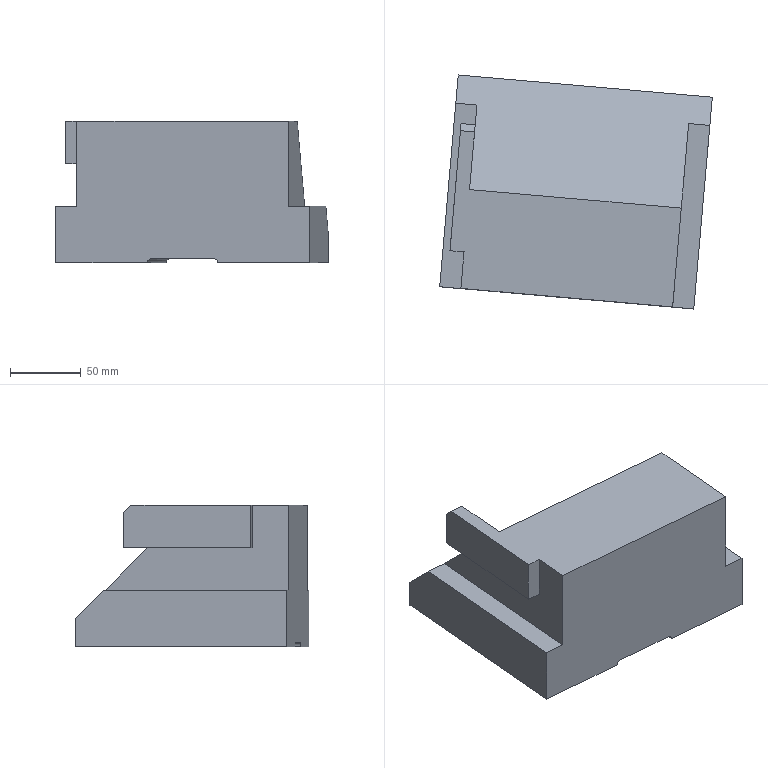Part | NX | features MAIN_BODY 2 | 1 solid | 21 faces | box 192.388 x 165.117 x 100 mm | volume 1948955 mm3 | plane 19 | cylinder 2 | commonest cylinder face diameters 6 x2
STEP:
#1=CARTESIAN_POINT('',(313.562,199.287,40.));
#2=VERTEX_POINT('',#1);
#3=CARTESIAN_POINT('',(306.154,114.611,40.));
#4=VERTEX_POINT('',#3);
#5=CARTESIAN_POINT('',(313.562,199.287,40.));
#6=CARTESIAN_POINT('',(311.093,171.062,40.));
#7=CARTESIAN_POINT('',(308.623,142.836,40.));
#8=CARTESIAN_POINT('',(306.154,114.611,40.));
#9=B_SPLINE_CURVE_WITH_KNOTS('',3,(#5,#6,#7,#8),.UNSPECIFIED.,.F.,.F.,(4,4),(0.,1.),.UNSPECIFIED.);
#10=EDGE_CURVE('',#2,#4,#9,.T.);
#11=ORIENTED_EDGE('',*,*,#10,.T.);
#12=CARTESIAN_POINT('',(316.116,113.739,40.));
#13=VERTEX_POINT('',#12);
#14=CARTESIAN_POINT('',(306.154,114.611,40.));
#15=CARTESIAN_POINT('',(309.475,114.32,40.));
#16=CARTESIAN_POINT('',(312.795,114.03,40.));
#17=CARTESIAN_POINT('',(316.116,113.739,40.));
#18=B_SPLINE_CURVE_WITH_KNOTS('',3,(#14,#15,#16,#17),.UNSPECIFIED.,.F.,.F.,(4,4),(0.,1.),.UNSPECIFIED.);
#19=EDGE_CURVE('',#4,#13,#18,.T.);
#20=ORIENTED_EDGE('',*,*,#19,.T.);
#21=CARTESIAN_POINT('',(313.862,87.98,40.));
#22=VERTEX_POINT('',#21);
#23=CARTESIAN_POINT('',(316.116,113.739,40.));
#24=CARTESIAN_POINT('',(315.365,105.153,40.));
#25=CARTESIAN_POINT('',(314.614,96.566,40.));
#26=CARTESIAN_POINT('',(313.862,87.98,40.));
#27=B_SPLINE_CURVE_WITH_KNOTS('',3,(#23,#24,#25,#26),.UNSPECIFIED.,.F.,.F.,(4,4),(0.,1.),.UNSPECIFIED.);
#28=EDGE_CURVE('',#13,#22,#27,.T.);
#29=ORIENTED_EDGE('',*,*,#28,.T.);
#30=CARTESIAN_POINT('',(463.291,74.907,40.));
#31=VERTEX_POINT('',#30);
#32=CARTESIAN_POINT('',(313.862,87.98,40.));
#33=CARTESIAN_POINT('',(363.672,83.622,40.));
#34=CARTESIAN_POINT('',(413.482,79.264,40.));
#35=CARTESIAN_POINT('',(463.291,74.907,40.));
#36=B_SPLINE_CURVE_WITH_KNOTS('',3,(#32,#33,#34,#35),.UNSPECIFIED.,.F.,.F.,(4,4),(0.,1.),.UNSPECIFIED.);
#37=EDGE_CURVE('',#22,#31,#36,.T.);
#38=ORIENTED_EDGE('',*,*,#37,.T.);
#39=CARTESIAN_POINT('',(469.392,144.64,40.));
#40=VERTEX_POINT('',#39);
#41=CARTESIAN_POINT('',(463.291,74.907,40.));
#42=CARTESIAN_POINT('',(465.325,98.151,40.));
#43=CARTESIAN_POINT('',(467.359,121.396,40.));
#44=CARTESIAN_POINT('',(469.392,144.64,40.));
#45=B_SPLINE_CURVE_WITH_KNOTS('',3,(#41,#42,#43,#44),.UNSPECIFIED.,.F.,.F.,(4,4),(0.,1.),.UNSPECIFIED.);
#46=EDGE_CURVE('',#31,#40,#45,.T.);
#47=ORIENTED_EDGE('',*,*,#46,.T.);
#48=CARTESIAN_POINT('',(319.963,157.714,40.));
#49=VERTEX_POINT('',#48);
#50=CARTESIAN_POINT('',(469.392,144.64,40.));
#51=CARTESIAN_POINT('',(419.583,148.998,40.));
#52=CARTESIAN_POINT('',(369.773,153.356,40.));
#53=CARTESIAN_POINT('',(319.963,157.714,40.));
#54=B_SPLINE_CURVE_WITH_KNOTS('',3,(#50,#51,#52,#53),.UNSPECIFIED.,.F.,.F.,(4,4),(0.,1.),.UNSPECIFIED.);
#55=EDGE_CURVE('',#40,#49,#54,.T.);
#56=ORIENTED_EDGE('',*,*,#55,.T.);
#57=CARTESIAN_POINT('',(323.524,198.416,40.));
#58=VERTEX_POINT('',#57);
#59=CARTESIAN_POINT('',(319.963,157.714,40.));
#60=CARTESIAN_POINT('',(321.15,171.281,40.));
#61=CARTESIAN_POINT('',(322.337,184.848,40.));
#62=CARTESIAN_POINT('',(323.524,198.416,40.));
#63=B_SPLINE_CURVE_WITH_KNOTS('',3,(#59,#60,#61,#62),.UNSPECIFIED.,.F.,.F.,(4,4),(0.,1.),.UNSPECIFIED.);
#64=EDGE_CURVE('',#49,#58,#63,.T.);
#65=ORIENTED_EDGE('',*,*,#64,.T.);
#66=CARTESIAN_POINT('',(323.524,198.416,40.));
#67=CARTESIAN_POINT('',(320.204,198.706,40.));
#68=CARTESIAN_POINT('',(316.883,198.997,40.));
#69=CARTESIAN_POINT('',(313.562,199.287,40.));
#70=B_SPLINE_CURVE_WITH_KNOTS('',3,(#66,#67,#68,#69),.UNSPECIFIED.,.F.,.F.,(4,4),(0.,1.),.UNSPECIFIED.);
#71=EDGE_CURVE('',#58,#2,#70,.T.);
#72=ORIENTED_EDGE('',*,*,#71,.T.);
#73=EDGE_LOOP('',(#11,#20,#29,#38,#47,#56,#65,#72));
#74=FACE_BOUND('',#73,.T.);
#75=CARTESIAN_POINT('',(388.427,137.097,40.));
#76=DIRECTION('',(0.,0.,1.));
#77=DIRECTION('',(-0.9962,0.08716,0.));
#78=AXIS2_PLACEMENT_3D('',#75,#76,#77);
#79=PLANE('',#78);
#80=ADVANCED_FACE('',(#74),#79,.T.);
#81=CARTESIAN_POINT('',(316.116,113.739,10.));
#82=VERTEX_POINT('',#81);
#83=CARTESIAN_POINT('',(316.116,113.739,10.));
#84=CARTESIAN_POINT('',(316.116,113.739,20.));
#85=CARTESIAN_POINT('',(316.116,113.739,30.));
#86=CARTESIAN_POINT('',(316.116,113.739,40.));
#87=B_SPLINE_CURVE_WITH_KNOTS('',3,(#83,#84,#85,#86),.UNSPECIFIED.,.F.,.F.,(4,4),(0.,1.),.UNSPECIFIED.);
#88=EDGE_CURVE('',#82,#13,#87,.T.);
#89=ORIENTED_EDGE('',*,*,#88,.T.);
#90=ORIENTED_EDGE('',*,*,#19,.F.);
#91=CARTESIAN_POINT('',(306.154,114.611,10.));
#92=VERTEX_POINT('',#91);
#93=CARTESIAN_POINT('',(306.154,114.611,40.));
#94=CARTESIAN_POINT('',(306.154,114.611,30.));
#95=CARTESIAN_POINT('',(306.154,114.611,20.));
#96=CARTESIAN_POINT('',(306.154,114.611,10.));
#97=B_SPLINE_CURVE_WITH_KNOTS('',3,(#93,#94,#95,#96),.UNSPECIFIED.,.F.,.F.,(4,4),(0.,1.),.UNSPECIFIED.);
#98=EDGE_CURVE('',#4,#92,#97,.T.);
#99=ORIENTED_EDGE('',*,*,#98,.T.);
#100=CARTESIAN_POINT('',(306.154,114.611,10.));
#101=CARTESIAN_POINT('',(309.475,114.32,10.));
#102=CARTESIAN_POINT('',(312.795,114.03,10.));
#103=CARTESIAN_POINT('',(316.116,113.739,10.));
#104=B_SPLINE_CURVE_WITH_KNOTS('',3,(#100,#101,#102,#103),.UNSPECIFIED.,.F.,.F.,(4,4),(0.,1.),.UNSPECIFIED.);
#105=EDGE_CURVE('',#92,#82,#104,.T.);
#106=ORIENTED_EDGE('',*,*,#105,.T.);
#107=EDGE_LOOP('',(#89,#90,#99,#106));
#108=FACE_BOUND('',#107,.T.);
#109=CARTESIAN_POINT('',(311.135,114.175,25.));
#110=DIRECTION('',(-0.08716,-0.9962,0.));
#111=DIRECTION('',(0.9962,-0.08716,0.));
#112=AXIS2_PLACEMENT_3D('',#109,#110,#111);
#113=PLANE('',#112);
#114=ADVANCED_FACE('',(#108),#113,.T.);
#115=CARTESIAN_POINT('',(313.998,204.268,10.));
#116=VERTEX_POINT('',#115);
#117=CARTESIAN_POINT('',(313.998,204.268,10.));
#118=CARTESIAN_POINT('',(311.383,174.383,10.));
#119=CARTESIAN_POINT('',(308.769,144.497,10.));
#120=CARTESIAN_POINT('',(306.154,114.611,10.));
#121=B_SPLINE_CURVE_WITH_KNOTS('',3,(#117,#118,#119,#120),.UNSPECIFIED.,.F.,.F.,(4,4),(0.,1.),.UNSPECIFIED.);
#122=EDGE_CURVE('',#116,#92,#121,.T.);
#123=ORIENTED_EDGE('',*,*,#122,.T.);
#124=ORIENTED_EDGE('',*,*,#98,.F.);
#125=ORIENTED_EDGE('',*,*,#10,.F.);
#126=CARTESIAN_POINT('',(313.998,204.268,35.));
#127=VERTEX_POINT('',#126);
#128=CARTESIAN_POINT('',(313.562,199.287,40.));
#129=CARTESIAN_POINT('',(313.708,200.948,38.333));
#130=CARTESIAN_POINT('',(313.853,202.608,36.667));
#131=CARTESIAN_POINT('',(313.998,204.268,35.));
#132=B_SPLINE_CURVE_WITH_KNOTS('',3,(#128,#129,#130,#131),.UNSPECIFIED.,.F.,.F.,(4,4),(0.,1.),.UNSPECIFIED.);
#133=EDGE_CURVE('',#2,#127,#132,.T.);
#134=ORIENTED_EDGE('',*,*,#133,.T.);
#135=CARTESIAN_POINT('',(313.998,204.268,35.));
#136=CARTESIAN_POINT('',(313.998,204.268,26.667));
#137=CARTESIAN_POINT('',(313.998,204.268,18.333));
#138=CARTESIAN_POINT('',(313.998,204.268,10.));
#139=B_SPLINE_CURVE_WITH_KNOTS('',3,(#135,#136,#137,#138),.UNSPECIFIED.,.F.,.F.,(4,4),(0.,1.),.UNSPECIFIED.);
#140=EDGE_CURVE('',#127,#116,#139,.T.);
#141=ORIENTED_EDGE('',*,*,#140,.T.);
#142=EDGE_LOOP('',(#123,#124,#125,#134,#141));
#143=FACE_BOUND('',#142,.T.);
#144=CARTESIAN_POINT('',(310.076,159.44,25.));
#145=DIRECTION('',(-0.9962,0.08716,0.));
#146=DIRECTION('',(-0.08716,-0.9962,0.));
#147=AXIS2_PLACEMENT_3D('',#144,#145,#146);
#148=PLANE('',#147);
#149=ADVANCED_FACE('',(#143),#148,.T.);
#150=CARTESIAN_POINT('',(323.96,203.397,35.));
#151=VERTEX_POINT('',#150);
#152=CARTESIAN_POINT('',(323.524,198.416,40.));
#153=CARTESIAN_POINT('',(323.669,200.076,38.333));
#154=CARTESIAN_POINT('',(323.815,201.737,36.667));
#155=CARTESIAN_POINT('',(323.96,203.397,35.));
#156=B_SPLINE_CURVE_WITH_KNOTS('',3,(#152,#153,#154,#155),.UNSPECIFIED.,.F.,.F.,(4,4),(0.,1.),.UNSPECIFIED.);
#157=EDGE_CURVE('',#58,#151,#156,.T.);
#158=ORIENTED_EDGE('',*,*,#157,.T.);
#159=CARTESIAN_POINT('',(323.96,203.397,35.));
#160=CARTESIAN_POINT('',(320.639,203.687,35.));
#161=CARTESIAN_POINT('',(317.319,203.978,35.));
#162=CARTESIAN_POINT('',(313.998,204.268,35.));
#163=B_SPLINE_CURVE_WITH_KNOTS('',3,(#159,#160,#161,#162),.UNSPECIFIED.,.F.,.F.,(4,4),(0.,1.),.UNSPECIFIED.);
#164=EDGE_CURVE('',#151,#127,#163,.T.);
#165=ORIENTED_EDGE('',*,*,#164,.T.);
#166=ORIENTED_EDGE('',*,*,#133,.F.);
#167=ORIENTED_EDGE('',*,*,#71,.F.);
#168=EDGE_LOOP('',(#158,#165,#166,#167));
#169=FACE_BOUND('',#168,.T.);
#170=CARTESIAN_POINT('',(318.761,201.342,37.5));
#171=DIRECTION('',(0.06163,0.7044,0.7071));
#172=DIRECTION('',(0.06163,0.7044,-0.7071));
#173=AXIS2_PLACEMENT_3D('',#170,#171,#172);
#174=PLANE('',#173);
#175=ADVANCED_FACE('',(#169),#174,.T.);
#176=ORIENTED_EDGE('',*,*,#157,.F.);
#177=ORIENTED_EDGE('',*,*,#64,.F.);
#178=CARTESIAN_POINT('',(322.578,187.599,10.));
#179=VERTEX_POINT('',#178);
#180=CARTESIAN_POINT('',(319.963,157.714,40.));
#181=CARTESIAN_POINT('',(320.835,167.675,30.));
#182=CARTESIAN_POINT('',(321.706,177.637,20.));
#183=CARTESIAN_POINT('',(322.578,187.599,10.));
#184=B_SPLINE_CURVE_WITH_KNOTS('',3,(#180,#181,#182,#183),.UNSPECIFIED.,.F.,.F.,(4,4),(0.,1.),.UNSPECIFIED.);
#185=EDGE_CURVE('',#49,#179,#184,.T.);
#186=ORIENTED_EDGE('',*,*,#185,.T.);
#187=CARTESIAN_POINT('',(323.96,203.397,10.));
#188=VERTEX_POINT('',#187);
#189=CARTESIAN_POINT('',(322.578,187.599,10.));
#190=CARTESIAN_POINT('',(323.039,192.865,10.));
#191=CARTESIAN_POINT('',(323.499,198.131,10.));
#192=CARTESIAN_POINT('',(323.96,203.397,10.));
#193=B_SPLINE_CURVE_WITH_KNOTS('',3,(#189,#190,#191,#192),.UNSPECIFIED.,.F.,.F.,(4,4),(0.,1.),.UNSPECIFIED.);
#194=EDGE_CURVE('',#179,#188,#193,.T.);
#195=ORIENTED_EDGE('',*,*,#194,.T.);
#196=CARTESIAN_POINT('',(323.96,203.397,10.));
#197=CARTESIAN_POINT('',(323.96,203.397,18.333));
#198=CARTESIAN_POINT('',(323.96,203.397,26.667));
#199=CARTESIAN_POINT('',(323.96,203.397,35.));
#200=B_SPLINE_CURVE_WITH_KNOTS('',3,(#196,#197,#198,#199),.UNSPECIFIED.,.F.,.F.,(4,4),(0.,1.),.UNSPECIFIED.);
#201=EDGE_CURVE('',#188,#151,#200,.T.);
#202=ORIENTED_EDGE('',*,*,#201,.T.);
#203=EDGE_LOOP('',(#176,#177,#186,#195,#202));
#204=FACE_BOUND('',#203,.T.);
#205=CARTESIAN_POINT('',(321.962,180.555,25.));
#206=DIRECTION('',(0.9962,-0.08716,0.));
#207=DIRECTION('',(0.08716,0.9962,0.));
#208=AXIS2_PLACEMENT_3D('',#205,#206,#207);
#209=PLANE('',#208);
#210=ADVANCED_FACE('',(#204),#209,.T.);
#211=CARTESIAN_POINT('',(491.308,223.028,-40.));
#212=VERTEX_POINT('',#211);
#213=CARTESIAN_POINT('',(311.993,238.716,-40.));
#214=VERTEX_POINT('',#213);
#215=CARTESIAN_POINT('',(491.308,223.028,-40.));
#216=CARTESIAN_POINT('',(431.536,228.258,-40.));
#217=CARTESIAN_POINT('',(371.764,233.487,-40.));
#218=CARTESIAN_POINT('',(311.993,238.716,-40.));
#219=B_SPLINE_CURVE_WITH_KNOTS('',3,(#215,#216,#217,#218),.UNSPECIFIED.,.F.,.F.,(4,4),(0.,1.),.UNSPECIFIED.);
#220=EDGE_CURVE('',#212,#214,#219,.T.);
#221=ORIENTED_EDGE('',*,*,#220,.T.);
#222=CARTESIAN_POINT('',(310.25,218.793,-20.));
#223=VERTEX_POINT('',#222);
#224=CARTESIAN_POINT('',(311.993,238.716,-40.));
#225=CARTESIAN_POINT('',(311.412,232.075,-33.333));
#226=CARTESIAN_POINT('',(310.831,225.434,-26.667));
#227=CARTESIAN_POINT('',(310.25,218.793,-20.));
#228=B_SPLINE_CURVE_WITH_KNOTS('',3,(#224,#225,#226,#227),.UNSPECIFIED.,.F.,.F.,(4,4),(0.,1.),.UNSPECIFIED.);
#229=EDGE_CURVE('',#214,#223,#228,.T.);
#230=ORIENTED_EDGE('',*,*,#229,.T.);
#231=CARTESIAN_POINT('',(325.193,217.485,-20.));
#232=VERTEX_POINT('',#231);
#233=CARTESIAN_POINT('',(310.25,218.793,-20.));
#234=CARTESIAN_POINT('',(315.231,218.357,-20.));
#235=CARTESIAN_POINT('',(320.212,217.921,-20.));
#236=CARTESIAN_POINT('',(325.193,217.485,-20.));
#237=B_SPLINE_CURVE_WITH_KNOTS('',3,(#233,#234,#235,#236),.UNSPECIFIED.,.F.,.F.,(4,4),(0.,1.),.UNSPECIFIED.);
#238=EDGE_CURVE('',#223,#232,#237,.T.);
#239=ORIENTED_EDGE('',*,*,#238,.T.);
#240=CARTESIAN_POINT('',(325.193,217.485,-20.));
#241=CARTESIAN_POINT('',(324.321,207.523,-10.));
#242=CARTESIAN_POINT('',(323.449,197.561,-0.000000002));
#243=CARTESIAN_POINT('',(322.578,187.599,10.));
#244=B_SPLINE_CURVE_WITH_KNOTS('',3,(#240,#241,#242,#243),.UNSPECIFIED.,.F.,.F.,(4,4),(0.,1.),.UNSPECIFIED.);
#245=EDGE_CURVE('',#232,#179,#244,.T.);
#246=ORIENTED_EDGE('',*,*,#245,.T.);
#247=ORIENTED_EDGE('',*,*,#185,.F.);
#248=ORIENTED_EDGE('',*,*,#55,.F.);
#249=CARTESIAN_POINT('',(474.622,204.412,-20.));
#250=VERTEX_POINT('',#249);
#251=CARTESIAN_POINT('',(469.392,144.64,40.));
#252=CARTESIAN_POINT('',(471.136,164.564,20.));
#253=CARTESIAN_POINT('',(472.879,184.488,-0.000000003));
#254=CARTESIAN_POINT('',(474.622,204.412,-20.));
#255=B_SPLINE_CURVE_WITH_KNOTS('',3,(#251,#252,#253,#254),.UNSPECIFIED.,.F.,.F.,(4,4),(0.,1.),.UNSPECIFIED.);
#256=EDGE_CURVE('',#40,#250,#255,.T.);
#257=ORIENTED_EDGE('',*,*,#256,.T.);
#258=CARTESIAN_POINT('',(489.565,203.105,-20.));
#259=VERTEX_POINT('',#258);
#260=CARTESIAN_POINT('',(474.622,204.412,-20.));
#261=CARTESIAN_POINT('',(479.603,203.976,-20.));
#262=CARTESIAN_POINT('',(484.584,203.54,-20.));
#263=CARTESIAN_POINT('',(489.565,203.105,-20.));
#264=B_SPLINE_CURVE_WITH_KNOTS('',3,(#260,#261,#262,#263),.UNSPECIFIED.,.F.,.F.,(4,4),(0.,1.),.UNSPECIFIED.);
#265=EDGE_CURVE('',#250,#259,#264,.T.);
#266=ORIENTED_EDGE('',*,*,#265,.T.);
#267=CARTESIAN_POINT('',(489.565,203.105,-20.));
#268=CARTESIAN_POINT('',(490.146,209.746,-26.667));
#269=CARTESIAN_POINT('',(490.727,216.387,-33.333));
#270=CARTESIAN_POINT('',(491.308,223.028,-40.));
#271=B_SPLINE_CURVE_WITH_KNOTS('',3,(#267,#268,#269,#270),.UNSPECIFIED.,.F.,.F.,(4,4),(0.,1.),.UNSPECIFIED.);
#272=EDGE_CURVE('',#259,#212,#271,.T.);
#273=ORIENTED_EDGE('',*,*,#272,.T.);
#274=EDGE_LOOP('',(#221,#230,#239,#246,#247,#248,#257,#266,#273));
#275=FACE_BOUND('',#274,.T.);
#276=CARTESIAN_POINT('',(398.164,191.025,-0.00000004));
#277=DIRECTION('',(0.06163,0.7044,0.7071));
#278=DIRECTION('',(0.06163,0.7044,-0.7071));
#279=AXIS2_PLACEMENT_3D('',#276,#277,#278);
#280=PLANE('',#279);
#281=ADVANCED_FACE('',(#275),#280,.T.);
#282=CARTESIAN_POINT('',(463.291,74.907,-20.));
#283=VERTEX_POINT('',#282);
#284=CARTESIAN_POINT('',(463.291,74.907,40.));
#285=CARTESIAN_POINT('',(463.291,74.907,20.));
#286=CARTESIAN_POINT('',(463.291,74.907,-0.000000003));
#287=CARTESIAN_POINT('',(463.291,74.907,-20.));
#288=B_SPLINE_CURVE_WITH_KNOTS('',3,(#284,#285,#286,#287),.UNSPECIFIED.,.F.,.F.,(4,4),(0.,1.),.UNSPECIFIED.);
#289=EDGE_CURVE('',#31,#283,#288,.T.);
#290=ORIENTED_EDGE('',*,*,#289,.T.);
#291=CARTESIAN_POINT('',(463.291,74.907,-20.));
#292=CARTESIAN_POINT('',(467.068,118.075,-20.));
#293=CARTESIAN_POINT('',(470.845,161.243,-20.));
#294=CARTESIAN_POINT('',(474.622,204.412,-20.));
#295=B_SPLINE_CURVE_WITH_KNOTS('',3,(#291,#292,#293,#294),.UNSPECIFIED.,.F.,.F.,(4,4),(0.,1.),.UNSPECIFIED.);
#296=EDGE_CURVE('',#283,#250,#295,.T.);
#297=ORIENTED_EDGE('',*,*,#296,.T.);
#298=ORIENTED_EDGE('',*,*,#256,.F.);
#299=ORIENTED_EDGE('',*,*,#46,.F.);
#300=EDGE_LOOP('',(#290,#297,#298,#299));
#301=FACE_BOUND('',#300,.T.);
#302=CARTESIAN_POINT('',(468.957,139.659,10.));
#303=DIRECTION('',(0.9962,-0.08716,0.));
#304=DIRECTION('',(0.08716,0.9962,0.));
#305=AXIS2_PLACEMENT_3D('',#302,#303,#304);
#306=PLANE('',#305);
#307=ADVANCED_FACE('',(#301),#306,.T.);
#308=CARTESIAN_POINT('',(298.919,89.287,-20.));
#309=VERTEX_POINT('',#308);
#310=CARTESIAN_POINT('',(298.919,89.287,-60.));
#311=VERTEX_POINT('',#310);
#312=CARTESIAN_POINT('',(298.919,89.287,-20.));
#313=CARTESIAN_POINT('',(298.919,89.287,-33.333));
#314=CARTESIAN_POINT('',(298.919,89.287,-46.667));
#315=CARTESIAN_POINT('',(298.919,89.287,-60.));
#316=B_SPLINE_CURVE_WITH_KNOTS('',3,(#312,#313,#314,#315),.UNSPECIFIED.,.F.,.F.,(4,4),(0.,1.),.UNSPECIFIED.);
#317=EDGE_CURVE('',#309,#311,#316,.T.);
#318=ORIENTED_EDGE('',*,*,#317,.T.);
#319=CARTESIAN_POINT('',(363.672,83.622,-60.));
#320=VERTEX_POINT('',#319);
#321=CARTESIAN_POINT('',(298.919,89.287,-60.));
#322=CARTESIAN_POINT('',(320.504,87.399,-60.));
#323=CARTESIAN_POINT('',(342.088,85.51,-60.));
#324=CARTESIAN_POINT('',(363.672,83.622,-60.));
#325=B_SPLINE_CURVE_WITH_KNOTS('',3,(#321,#322,#323,#324),.UNSPECIFIED.,.F.,.F.,(4,4),(0.,1.),.UNSPECIFIED.);
#326=EDGE_CURVE('',#311,#320,#325,.T.);
#327=ORIENTED_EDGE('',*,*,#326,.T.);
#328=CARTESIAN_POINT('',(366.661,83.361,-57.));
#329=VERTEX_POINT('',#328);
#330=CARTESIAN_POINT('',(363.672,83.622,-60.));
#331=CARTESIAN_POINT('',(363.674,83.622,-59.87));
#332=CARTESIAN_POINT('',(363.68,83.621,-59.72));
#333=CARTESIAN_POINT('',(363.74,83.616,-59.309));
#334=CARTESIAN_POINT('',(363.938,83.599,-58.663));
#335=CARTESIAN_POINT('',(364.49,83.551,-57.822));
#336=CARTESIAN_POINT('',(365.329,83.477,-57.267));
#337=CARTESIAN_POINT('',(365.972,83.421,-57.068));
#338=CARTESIAN_POINT('',(366.382,83.385,-57.008));
#339=CARTESIAN_POINT('',(366.53,83.372,-57.004));
#340=CARTESIAN_POINT('',(366.661,83.361,-57.));
#341=B_SPLINE_CURVE_WITH_KNOTS('',3,(#330,#331,#332,#333,#334,#335,#336,#337,#338,#339,#340),.UNSPECIFIED.,.F.,.F.,(4,1,1,1,1,1,1,1,4),(0.,0.0625,0.125,0.25,0.5,0.75,0.875,0.9375,1.),.UNSPECIFIED.);
#342=EDGE_CURVE('',#320,#329,#341,.T.);
#343=ORIENTED_EDGE('',*,*,#342,.T.);
#344=CARTESIAN_POINT('',(410.493,79.526,-57.));
#345=VERTEX_POINT('',#344);
#346=CARTESIAN_POINT('',(366.661,83.361,-57.));
#347=CARTESIAN_POINT('',(381.271,82.082,-57.));
#348=CARTESIAN_POINT('',(395.882,80.804,-57.));
#349=CARTESIAN_POINT('',(410.493,79.526,-57.));
#350=B_SPLINE_CURVE_WITH_KNOTS('',3,(#346,#347,#348,#349),.UNSPECIFIED.,.F.,.F.,(4,4),(0.,1.),.UNSPECIFIED.);
#351=EDGE_CURVE('',#329,#345,#350,.T.);
#352=ORIENTED_EDGE('',*,*,#351,.T.);
#353=CARTESIAN_POINT('',(413.482,79.264,-60.));
#354=VERTEX_POINT('',#353);
#355=CARTESIAN_POINT('',(410.493,79.526,-57.));
#356=CARTESIAN_POINT('',(410.623,79.514,-57.002));
#357=CARTESIAN_POINT('',(410.772,79.501,-57.008));
#358=CARTESIAN_POINT('',(411.182,79.466,-57.068));
#359=CARTESIAN_POINT('',(411.825,79.409,-57.267));
#360=CARTESIAN_POINT('',(412.663,79.336,-57.821));
#361=CARTESIAN_POINT('',(413.216,79.288,-58.663));
#362=CARTESIAN_POINT('',(413.414,79.27,-59.308));
#363=CARTESIAN_POINT('',(413.474,79.265,-59.721));
#364=CARTESIAN_POINT('',(413.478,79.265,-59.869));
#365=CARTESIAN_POINT('',(413.482,79.264,-60.));
#366=B_SPLINE_CURVE_WITH_KNOTS('',3,(#355,#356,#357,#358,#359,#360,#361,#362,#363,#364,#365),.UNSPECIFIED.,.F.,.F.,(4,1,1,1,1,1,1,1,4),(0.,0.0625,0.125,0.25,0.5,0.75,0.875,0.9375,1.),.UNSPECIFIED.);
#367=EDGE_CURVE('',#345,#354,#366,.T.);
#368=ORIENTED_EDGE('',*,*,#367,.T.);
#369=CARTESIAN_POINT('',(478.234,73.599,-60.));
#370=VERTEX_POINT('',#369);
#371=CARTESIAN_POINT('',(413.482,79.264,-60.));
#372=CARTESIAN_POINT('',(435.066,77.376,-60.));
#373=CARTESIAN_POINT('',(456.65,75.488,-60.));
#374=CARTESIAN_POINT('',(478.234,73.599,-60.));
#375=B_SPLINE_CURVE_WITH_KNOTS('',3,(#371,#372,#373,#374),.UNSPECIFIED.,.F.,.F.,(4,4),(0.,1.),.UNSPECIFIED.);
#376=EDGE_CURVE('',#354,#370,#375,.T.);
#377=ORIENTED_EDGE('',*,*,#376,.T.);
#378=CARTESIAN_POINT('',(478.234,73.599,-20.));
#379=VERTEX_POINT('',#378);
#380=CARTESIAN_POINT('',(478.234,73.599,-60.));
#381=CARTESIAN_POINT('',(478.234,73.599,-46.667));
#382=CARTESIAN_POINT('',(478.234,73.599,-33.333));
#383=CARTESIAN_POINT('',(478.234,73.599,-20.));
#384=B_SPLINE_CURVE_WITH_KNOTS('',3,(#380,#381,#382,#383),.UNSPECIFIED.,.F.,.F.,(4,4),(0.,1.),.UNSPECIFIED.);
#385=EDGE_CURVE('',#370,#379,#384,.T.);
#386=ORIENTED_EDGE('',*,*,#385,.T.);
#387=CARTESIAN_POINT('',(478.234,73.599,-20.));
#388=CARTESIAN_POINT('',(473.253,74.035,-20.));
#389=CARTESIAN_POINT('',(468.272,74.471,-20.));
#390=CARTESIAN_POINT('',(463.291,74.907,-20.));
#391=B_SPLINE_CURVE_WITH_KNOTS('',3,(#387,#388,#389,#390),.UNSPECIFIED.,.F.,.F.,(4,4),(0.,1.),.UNSPECIFIED.);
#392=EDGE_CURVE('',#379,#283,#391,.T.);
#393=ORIENTED_EDGE('',*,*,#392,.T.);
#394=ORIENTED_EDGE('',*,*,#289,.F.);
#395=ORIENTED_EDGE('',*,*,#37,.F.);
#396=CARTESIAN_POINT('',(313.862,87.98,-20.));
#397=VERTEX_POINT('',#396);
#398=CARTESIAN_POINT('',(313.862,87.98,40.));
#399=CARTESIAN_POINT('',(313.862,87.98,20.));
#400=CARTESIAN_POINT('',(313.862,87.98,-0.000000003));
#401=CARTESIAN_POINT('',(313.862,87.98,-20.));
#402=B_SPLINE_CURVE_WITH_KNOTS('',3,(#398,#399,#400,#401),.UNSPECIFIED.,.F.,.F.,(4,4),(0.,1.),.UNSPECIFIED.);
#403=EDGE_CURVE('',#22,#397,#402,.T.);
#404=ORIENTED_EDGE('',*,*,#403,.T.);
#405=CARTESIAN_POINT('',(313.862,87.98,-20.));
#406=CARTESIAN_POINT('',(308.881,88.416,-20.));
#407=CARTESIAN_POINT('',(303.9,88.851,-20.));
#408=CARTESIAN_POINT('',(298.919,89.287,-20.));
#409=B_SPLINE_CURVE_WITH_KNOTS('',3,(#405,#406,#407,#408),.UNSPECIFIED.,.F.,.F.,(4,4),(0.,1.),.UNSPECIFIED.);
#410=EDGE_CURVE('',#397,#309,#409,.T.);
#411=ORIENTED_EDGE('',*,*,#410,.T.);
#412=EDGE_LOOP('',(#318,#327,#343,#352,#368,#377,#386,#393,#394,#395,#404,#411));
#413=FACE_BOUND('',#412,.T.);
#414=CARTESIAN_POINT('',(388.577,81.443,-10.));
#415=DIRECTION('',(-0.08716,-0.9962,0.));
#416=DIRECTION('',(0.9962,-0.08716,0.));
#417=AXIS2_PLACEMENT_3D('',#414,#415,#416);
#418=PLANE('',#417);
#419=ADVANCED_FACE('',(#413),#418,.T.);
#420=ORIENTED_EDGE('',*,*,#28,.F.);
#421=ORIENTED_EDGE('',*,*,#88,.F.);
#422=CARTESIAN_POINT('',(316.116,113.739,10.));
#423=CARTESIAN_POINT('',(318.27,138.359,10.));
#424=CARTESIAN_POINT('',(320.424,162.979,10.));
#425=CARTESIAN_POINT('',(322.578,187.599,10.));
#426=B_SPLINE_CURVE_WITH_KNOTS('',3,(#422,#423,#424,#425),.UNSPECIFIED.,.F.,.F.,(4,4),(0.,1.),.UNSPECIFIED.);
#427=EDGE_CURVE('',#82,#179,#426,.T.);
#428=ORIENTED_EDGE('',*,*,#427,.T.);
#429=ORIENTED_EDGE('',*,*,#245,.F.);
#430=CARTESIAN_POINT('',(325.193,217.485,-20.));
#431=CARTESIAN_POINT('',(321.416,174.317,-20.));
#432=CARTESIAN_POINT('',(317.639,131.148,-20.));
#433=CARTESIAN_POINT('',(313.862,87.98,-20.));
#434=B_SPLINE_CURVE_WITH_KNOTS('',3,(#430,#431,#432,#433),.UNSPECIFIED.,.F.,.F.,(4,4),(0.,1.),.UNSPECIFIED.);
#435=EDGE_CURVE('',#232,#397,#434,.T.);
#436=ORIENTED_EDGE('',*,*,#435,.T.);
#437=ORIENTED_EDGE('',*,*,#403,.F.);
#438=EDGE_LOOP('',(#420,#421,#428,#429,#436,#437));
#439=FACE_BOUND('',#438,.T.);
#440=CARTESIAN_POINT('',(319.527,152.733,10.));
#441=DIRECTION('',(-0.9962,0.08716,0.));
#442=DIRECTION('',(-0.08716,-0.9962,0.));
#443=AXIS2_PLACEMENT_3D('',#440,#441,#442);
#444=PLANE('',#443);
#445=ADVANCED_FACE('',(#439),#444,.T.);
#446=ORIENTED_EDGE('',*,*,#427,.F.);
#447=ORIENTED_EDGE('',*,*,#105,.F.);
#448=ORIENTED_EDGE('',*,*,#122,.F.);
#449=CARTESIAN_POINT('',(313.998,204.268,10.));
#450=CARTESIAN_POINT('',(317.319,203.978,10.));
#451=CARTESIAN_POINT('',(320.639,203.687,10.));
#452=CARTESIAN_POINT('',(323.96,203.397,10.));
#453=B_SPLINE_CURVE_WITH_KNOTS('',3,(#449,#450,#451,#452),.UNSPECIFIED.,.F.,.F.,(4,4),(0.,1.),.UNSPECIFIED.);
#454=EDGE_CURVE('',#116,#188,#453,.T.);
#455=ORIENTED_EDGE('',*,*,#454,.T.);
#456=ORIENTED_EDGE('',*,*,#194,.F.);
#457=EDGE_LOOP('',(#446,#447,#448,#455,#456));
#458=FACE_BOUND('',#457,.T.);
#459=CARTESIAN_POINT('',(315.057,159.004,10.));
#460=DIRECTION('',(0.,0.,-1.));
#461=DIRECTION('',(0.9962,-0.08716,0.));
#462=AXIS2_PLACEMENT_3D('',#459,#460,#461);
#463=PLANE('',#462);
#464=ADVANCED_FACE('',(#458),#463,.T.);
#465=ORIENTED_EDGE('',*,*,#201,.F.);
#466=ORIENTED_EDGE('',*,*,#454,.F.);
#467=ORIENTED_EDGE('',*,*,#140,.F.);
#468=ORIENTED_EDGE('',*,*,#164,.F.);
#469=EDGE_LOOP('',(#465,#466,#467,#468));
#470=FACE_BOUND('',#469,.T.);
#471=CARTESIAN_POINT('',(318.979,203.833,22.5));
#472=DIRECTION('',(0.08716,0.9962,0.));
#473=DIRECTION('',(-0.9962,0.08716,0.));
#474=AXIS2_PLACEMENT_3D('',#471,#472,#473);
#475=PLANE('',#474);
#476=ADVANCED_FACE('',(#470),#475,.T.);
#477=CARTESIAN_POINT('',(311.993,238.716,-60.));
#478=VERTEX_POINT('',#477);
#479=CARTESIAN_POINT('',(311.993,238.716,-60.));
#480=CARTESIAN_POINT('',(307.635,188.907,-60.));
#481=CARTESIAN_POINT('',(303.277,139.097,-60.));
#482=CARTESIAN_POINT('',(298.919,89.287,-60.));
#483=B_SPLINE_CURVE_WITH_KNOTS('',3,(#479,#480,#481,#482),.UNSPECIFIED.,.F.,.F.,(4,4),(0.,1.),.UNSPECIFIED.);
#484=EDGE_CURVE('',#478,#311,#483,.T.);
#485=ORIENTED_EDGE('',*,*,#484,.T.);
#486=ORIENTED_EDGE('',*,*,#317,.F.);
#487=CARTESIAN_POINT('',(298.919,89.287,-20.));
#488=CARTESIAN_POINT('',(302.696,132.456,-20.));
#489=CARTESIAN_POINT('',(306.473,175.624,-20.));
#490=CARTESIAN_POINT('',(310.25,218.793,-20.));
#491=B_SPLINE_CURVE_WITH_KNOTS('',3,(#487,#488,#489,#490),.UNSPECIFIED.,.F.,.F.,(4,4),(0.,1.),.UNSPECIFIED.);
#492=EDGE_CURVE('',#309,#223,#491,.T.);
#493=ORIENTED_EDGE('',*,*,#492,.T.);
#494=ORIENTED_EDGE('',*,*,#229,.F.);
#495=CARTESIAN_POINT('',(311.993,238.716,-40.));
#496=CARTESIAN_POINT('',(311.993,238.716,-46.667));
#497=CARTESIAN_POINT('',(311.993,238.716,-53.333));
#498=CARTESIAN_POINT('',(311.993,238.716,-60.));
#499=B_SPLINE_CURVE_WITH_KNOTS('',3,(#495,#496,#497,#498),.UNSPECIFIED.,.F.,.F.,(4,4),(0.,1.),.UNSPECIFIED.);
#500=EDGE_CURVE('',#214,#478,#499,.T.);
#501=ORIENTED_EDGE('',*,*,#500,.T.);
#502=EDGE_LOOP('',(#485,#486,#493,#494,#501));
#503=FACE_BOUND('',#502,.T.);
#504=CARTESIAN_POINT('',(305.456,164.002,-40.));
#505=DIRECTION('',(-0.9962,0.08716,0.));
#506=DIRECTION('',(-0.08716,-0.9962,0.));
#507=AXIS2_PLACEMENT_3D('',#504,#505,#506);
#508=PLANE('',#507);
#509=ADVANCED_FACE('',(#503),#508,.T.);
#510=CARTESIAN_POINT('',(426.555,228.694,-60.));
#511=VERTEX_POINT('',#510);
#512=CARTESIAN_POINT('',(423.567,228.955,-57.));
#513=VERTEX_POINT('',#512);
#514=CARTESIAN_POINT('',(426.555,228.694,-60.));
#515=CARTESIAN_POINT('',(426.553,228.694,-59.87));
#516=CARTESIAN_POINT('',(426.547,228.694,-59.72));
#517=CARTESIAN_POINT('',(426.488,228.699,-59.309));
#518=CARTESIAN_POINT('',(426.29,228.717,-58.663));
#519=CARTESIAN_POINT('',(425.737,228.765,-57.822));
#520=CARTESIAN_POINT('',(424.899,228.838,-57.267));
#521=CARTESIAN_POINT('',(424.255,228.895,-57.068));
#522=CARTESIAN_POINT('',(423.845,228.931,-57.008));
#523=CARTESIAN_POINT('',(423.697,228.944,-57.004));
#524=CARTESIAN_POINT('',(423.567,228.955,-57.));
#525=B_SPLINE_CURVE_WITH_KNOTS('',3,(#514,#515,#516,#517,#518,#519,#520,#521,#522,#523,#524),.UNSPECIFIED.,.F.,.F.,(4,1,1,1,1,1,1,1,4),(0.,0.0625,0.125,0.25,0.5,0.75,0.875,0.9375,1.),.UNSPECIFIED.);
#526=EDGE_CURVE('',#511,#513,#525,.T.);
#527=ORIENTED_EDGE('',*,*,#526,.T.);
#528=CARTESIAN_POINT('',(379.734,232.79,-57.));
#529=VERTEX_POINT('',#528);
#530=CARTESIAN_POINT('',(423.567,228.955,-57.));
#531=CARTESIAN_POINT('',(408.956,230.233,-57.));
#532=CARTESIAN_POINT('',(394.345,231.512,-57.));
#533=CARTESIAN_POINT('',(379.734,232.79,-57.));
#534=B_SPLINE_CURVE_WITH_KNOTS('',3,(#530,#531,#532,#533),.UNSPECIFIED.,.F.,.F.,(4,4),(0.,1.),.UNSPECIFIED.);
#535=EDGE_CURVE('',#513,#529,#534,.T.);
#536=ORIENTED_EDGE('',*,*,#535,.T.);
#537=CARTESIAN_POINT('',(376.745,233.051,-60.));
#538=VERTEX_POINT('',#537);
#539=CARTESIAN_POINT('',(379.734,232.79,-57.));
#540=CARTESIAN_POINT('',(379.604,232.801,-57.002));
#541=CARTESIAN_POINT('',(379.455,232.814,-57.008));
#542=CARTESIAN_POINT('',(379.046,232.85,-57.068));
#543=CARTESIAN_POINT('',(378.402,232.906,-57.267));
#544=CARTESIAN_POINT('',(377.564,232.98,-57.821));
#545=CARTESIAN_POINT('',(377.011,233.028,-58.663));
#546=CARTESIAN_POINT('',(376.813,233.045,-59.308));
#547=CARTESIAN_POINT('',(376.753,233.051,-59.721));
#548=CARTESIAN_POINT('',(376.749,233.051,-59.869));
#549=CARTESIAN_POINT('',(376.745,233.051,-60.));
#550=B_SPLINE_CURVE_WITH_KNOTS('',3,(#539,#540,#541,#542,#543,#544,#545,#546,#547,#548,#549),.UNSPECIFIED.,.F.,.F.,(4,1,1,1,1,1,1,1,4),(0.,0.0625,0.125,0.25,0.5,0.75,0.875,0.9375,1.),.UNSPECIFIED.);
#551=EDGE_CURVE('',#529,#538,#550,.T.);
#552=ORIENTED_EDGE('',*,*,#551,.T.);
#553=CARTESIAN_POINT('',(376.745,233.051,-60.));
#554=CARTESIAN_POINT('',(355.161,234.94,-60.));
#555=CARTESIAN_POINT('',(333.577,236.828,-60.));
#556=CARTESIAN_POINT('',(311.993,238.716,-60.));
#557=B_SPLINE_CURVE_WITH_KNOTS('',3,(#553,#554,#555,#556),.UNSPECIFIED.,.F.,.F.,(4,4),(0.,1.),.UNSPECIFIED.);
#558=EDGE_CURVE('',#538,#478,#557,.T.);
#559=ORIENTED_EDGE('',*,*,#558,.T.);
#560=ORIENTED_EDGE('',*,*,#500,.F.);
#561=ORIENTED_EDGE('',*,*,#220,.F.);
#562=CARTESIAN_POINT('',(491.308,223.028,-60.));
#563=VERTEX_POINT('',#562);
#564=CARTESIAN_POINT('',(491.308,223.028,-40.));
#565=CARTESIAN_POINT('',(491.308,223.028,-46.667));
#566=CARTESIAN_POINT('',(491.308,223.028,-53.333));
#567=CARTESIAN_POINT('',(491.308,223.028,-60.));
#568=B_SPLINE_CURVE_WITH_KNOTS('',3,(#564,#565,#566,#567),.UNSPECIFIED.,.F.,.F.,(4,4),(0.,1.),.UNSPECIFIED.);
#569=EDGE_CURVE('',#212,#563,#568,.T.);
#570=ORIENTED_EDGE('',*,*,#569,.T.);
#571=CARTESIAN_POINT('',(491.308,223.028,-60.));
#572=CARTESIAN_POINT('',(469.724,224.917,-60.));
#573=CARTESIAN_POINT('',(448.139,226.805,-60.));
#574=CARTESIAN_POINT('',(426.555,228.694,-60.));
#575=B_SPLINE_CURVE_WITH_KNOTS('',3,(#571,#572,#573,#574),.UNSPECIFIED.,.F.,.F.,(4,4),(0.,1.),.UNSPECIFIED.);
#576=EDGE_CURVE('',#563,#511,#575,.T.);
#577=ORIENTED_EDGE('',*,*,#576,.T.);
#578=EDGE_LOOP('',(#527,#536,#552,#559,#560,#561,#570,#577));
#579=FACE_BOUND('',#578,.T.);
#580=CARTESIAN_POINT('',(401.65,230.872,-50.));
#581=DIRECTION('',(0.08716,0.9962,0.));
#582=DIRECTION('',(-0.9962,0.08716,0.));
#583=AXIS2_PLACEMENT_3D('',#580,#581,#582);
#584=PLANE('',#583);
#585=ADVANCED_FACE('',(#579),#584,.T.);
#586=ORIENTED_EDGE('',*,*,#569,.F.);
#587=ORIENTED_EDGE('',*,*,#272,.F.);
#588=CARTESIAN_POINT('',(489.565,203.105,-20.));
#589=CARTESIAN_POINT('',(485.788,159.936,-20.));
#590=CARTESIAN_POINT('',(482.011,116.768,-20.));
#591=CARTESIAN_POINT('',(478.234,73.599,-20.));
#592=B_SPLINE_CURVE_WITH_KNOTS('',3,(#588,#589,#590,#591),.UNSPECIFIED.,.F.,.F.,(4,4),(0.,1.),.UNSPECIFIED.);
#593=EDGE_CURVE('',#259,#379,#592,.T.);
#594=ORIENTED_EDGE('',*,*,#593,.T.);
#595=ORIENTED_EDGE('',*,*,#385,.F.);
#596=CARTESIAN_POINT('',(478.234,73.599,-60.));
#597=CARTESIAN_POINT('',(482.592,123.409,-60.));
#598=CARTESIAN_POINT('',(486.95,173.219,-60.));
#599=CARTESIAN_POINT('',(491.308,223.028,-60.));
#600=B_SPLINE_CURVE_WITH_KNOTS('',3,(#596,#597,#598,#599),.UNSPECIFIED.,.F.,.F.,(4,4),(0.,1.),.UNSPECIFIED.);
#601=EDGE_CURVE('',#370,#563,#600,.T.);
#602=ORIENTED_EDGE('',*,*,#601,.T.);
#603=EDGE_LOOP('',(#586,#587,#594,#595,#602));
#604=FACE_BOUND('',#603,.T.);
#605=CARTESIAN_POINT('',(484.771,148.314,-40.));
#606=DIRECTION('',(0.9962,-0.08716,0.));
#607=DIRECTION('',(0.08716,0.9962,0.));
#608=AXIS2_PLACEMENT_3D('',#605,#606,#607);
#609=PLANE('',#608);
#610=ADVANCED_FACE('',(#604),#609,.T.);
#611=ORIENTED_EDGE('',*,*,#392,.F.);
#612=ORIENTED_EDGE('',*,*,#593,.F.);
#613=ORIENTED_EDGE('',*,*,#265,.F.);
#614=ORIENTED_EDGE('',*,*,#296,.F.);
#615=EDGE_LOOP('',(#611,#612,#613,#614));
#616=FACE_BOUND('',#615,.T.);
#617=CARTESIAN_POINT('',(476.428,139.006,-20.));
#618=DIRECTION('',(0.,0.,1.));
#619=DIRECTION('',(-0.9962,0.08716,0.));
#620=AXIS2_PLACEMENT_3D('',#617,#618,#619);
#621=PLANE('',#620);
#622=ADVANCED_FACE('',(#616),#621,.T.);
#623=ORIENTED_EDGE('',*,*,#410,.F.);
#624=ORIENTED_EDGE('',*,*,#435,.F.);
#625=ORIENTED_EDGE('',*,*,#238,.F.);
#626=ORIENTED_EDGE('',*,*,#492,.F.);
#627=EDGE_LOOP('',(#623,#624,#625,#626));
#628=FACE_BOUND('',#627,.T.);
#629=CARTESIAN_POINT('',(312.056,153.386,-20.));
#630=DIRECTION('',(0.,0.,1.));
#631=DIRECTION('',(-0.9962,0.08716,0.));
#632=AXIS2_PLACEMENT_3D('',#629,#630,#631);
#633=PLANE('',#632);
#634=ADVANCED_FACE('',(#628),#633,.T.);
#635=ORIENTED_EDGE('',*,*,#484,.F.);
#636=ORIENTED_EDGE('',*,*,#558,.F.);
#637=CARTESIAN_POINT('',(376.745,233.051,-60.));
#638=CARTESIAN_POINT('',(372.388,183.242,-60.));
#639=CARTESIAN_POINT('',(368.03,133.432,-60.));
#640=CARTESIAN_POINT('',(363.672,83.622,-60.));
#641=B_SPLINE_CURVE_WITH_KNOTS('',3,(#637,#638,#639,#640),.UNSPECIFIED.,.F.,.F.,(4,4),(0.,1.),.UNSPECIFIED.);
#642=EDGE_CURVE('',#538,#320,#641,.T.);
#643=ORIENTED_EDGE('',*,*,#642,.T.);
#644=ORIENTED_EDGE('',*,*,#326,.F.);
#645=EDGE_LOOP('',(#635,#636,#643,#644));
#646=FACE_BOUND('',#645,.T.);
#647=CARTESIAN_POINT('',(337.832,161.169,-60.));
#648=DIRECTION('',(0.,0.,-1.));
#649=DIRECTION('',(0.9962,-0.08716,0.));
#650=AXIS2_PLACEMENT_3D('',#647,#648,#649);
#651=PLANE('',#650);
#652=ADVANCED_FACE('',(#646),#651,.T.);
#653=ORIENTED_EDGE('',*,*,#601,.F.);
#654=ORIENTED_EDGE('',*,*,#376,.F.);
#655=CARTESIAN_POINT('',(413.482,79.264,-60.));
#656=CARTESIAN_POINT('',(417.84,129.074,-60.));
#657=CARTESIAN_POINT('',(422.197,178.884,-60.));
#658=CARTESIAN_POINT('',(426.555,228.694,-60.));
#659=B_SPLINE_CURVE_WITH_KNOTS('',3,(#655,#656,#657,#658),.UNSPECIFIED.,.F.,.F.,(4,4),(0.,1.),.UNSPECIFIED.);
#660=EDGE_CURVE('',#354,#511,#659,.T.);
#661=ORIENTED_EDGE('',*,*,#660,.T.);
#662=ORIENTED_EDGE('',*,*,#576,.F.);
#663=EDGE_LOOP('',(#653,#654,#661,#662));
#664=FACE_BOUND('',#663,.T.);
#665=CARTESIAN_POINT('',(452.395,151.146,-60.));
#666=DIRECTION('',(0.,0.,-1.));
#667=DIRECTION('',(0.9962,-0.08716,0.));
#668=AXIS2_PLACEMENT_3D('',#665,#666,#667);
#669=PLANE('',#668);
#670=ADVANCED_FACE('',(#664),#669,.T.);
#671=ORIENTED_EDGE('',*,*,#367,.F.);
#672=CARTESIAN_POINT('',(423.567,228.955,-57.));
#673=CARTESIAN_POINT('',(419.209,179.145,-57.));
#674=CARTESIAN_POINT('',(414.851,129.336,-57.));
#675=CARTESIAN_POINT('',(410.493,79.526,-57.));
#676=B_SPLINE_CURVE_WITH_KNOTS('',3,(#672,#673,#674,#675),.UNSPECIFIED.,.F.,.F.,(4,4),(0.,1.),.UNSPECIFIED.);
#677=EDGE_CURVE('',#345,#513,#676,.F.);
#678=ORIENTED_EDGE('',*,*,#677,.T.);
#679=ORIENTED_EDGE('',*,*,#526,.F.);
#680=ORIENTED_EDGE('',*,*,#660,.F.);
#681=EDGE_LOOP('',(#671,#678,#679,#680));
#682=FACE_BOUND('',#681,.T.);
#683=CARTESIAN_POINT('',(413.108,109.412,-60.));
#684=DIRECTION('',(0.08716,0.9962,0.));
#685=DIRECTION('',(-0.9962,0.08716,0.));
#686=AXIS2_PLACEMENT_3D('',#683,#684,#685);
#687=CYLINDRICAL_SURFACE('',#686,3.);
#688=ADVANCED_FACE('',(#682),#687,.F.);
#689=ORIENTED_EDGE('',*,*,#351,.F.);
#690=CARTESIAN_POINT('',(366.661,83.361,-57.));
#691=CARTESIAN_POINT('',(371.018,133.17,-57.));
#692=CARTESIAN_POINT('',(375.376,182.98,-57.));
#693=CARTESIAN_POINT('',(379.734,232.79,-57.));
#694=B_SPLINE_CURVE_WITH_KNOTS('',3,(#690,#691,#692,#693),.UNSPECIFIED.,.F.,.F.,(4,4),(0.,1.),.UNSPECIFIED.);
#695=EDGE_CURVE('',#329,#529,#694,.T.);
#696=ORIENTED_EDGE('',*,*,#695,.T.);
#697=ORIENTED_EDGE('',*,*,#535,.F.);
#698=ORIENTED_EDGE('',*,*,#677,.F.);
#699=EDGE_LOOP('',(#689,#696,#697,#698));
#700=FACE_BOUND('',#699,.T.);
#701=CARTESIAN_POINT('',(395.114,156.158,-57.));
#702=DIRECTION('',(0.,0.,-1.));
#703=DIRECTION('',(0.9962,-0.08716,0.));
#704=AXIS2_PLACEMENT_3D('',#701,#702,#703);
#705=PLANE('',#704);
#706=ADVANCED_FACE('',(#700),#705,.T.);
#707=ORIENTED_EDGE('',*,*,#342,.F.);
#708=ORIENTED_EDGE('',*,*,#642,.F.);
#709=ORIENTED_EDGE('',*,*,#551,.F.);
#710=ORIENTED_EDGE('',*,*,#695,.F.);
#711=EDGE_LOOP('',(#707,#708,#709,#710));
#712=FACE_BOUND('',#711,.T.);
#713=CARTESIAN_POINT('',(369.275,113.246,-60.));
#714=DIRECTION('',(0.08716,0.9962,0.));
#715=DIRECTION('',(-0.9962,0.08716,0.));
#716=AXIS2_PLACEMENT_3D('',#713,#714,#715);
#717=CYLINDRICAL_SURFACE('',#716,3.);
#718=ADVANCED_FACE('',(#712),#717,.F.);
#719=CLOSED_SHELL('',(#80,#114,#149,#175,#210,#281,#307,#419,#445,#464,#476,#509,#585,#610,#622,#634,#652,#670,#688,#706,#718));
#720=MANIFOLD_SOLID_BREP('',#719);
#721=(LENGTH_UNIT()NAMED_UNIT(*)SI_UNIT(.MILLI.,.METRE.));
#722=UNCERTAINTY_MEASURE_WITH_UNIT(LENGTH_MEASURE(0.0508),#721,'','');
#723=(NAMED_UNIT(*)PLANE_ANGLE_UNIT()SI_UNIT($,.RADIAN.));
#724=(NAMED_UNIT(*)SI_UNIT($,.STERADIAN.)SOLID_ANGLE_UNIT());
#725=(GEOMETRIC_REPRESENTATION_CONTEXT(3)GLOBAL_UNCERTAINTY_ASSIGNED_CONTEXT((#722))GLOBAL_UNIT_ASSIGNED_CONTEXT((#721,#723,#724))REPRESENTATION_CONTEXT('',''));
#726=ADVANCED_BREP_SHAPE_REPRESENTATION('',(#720),#725);